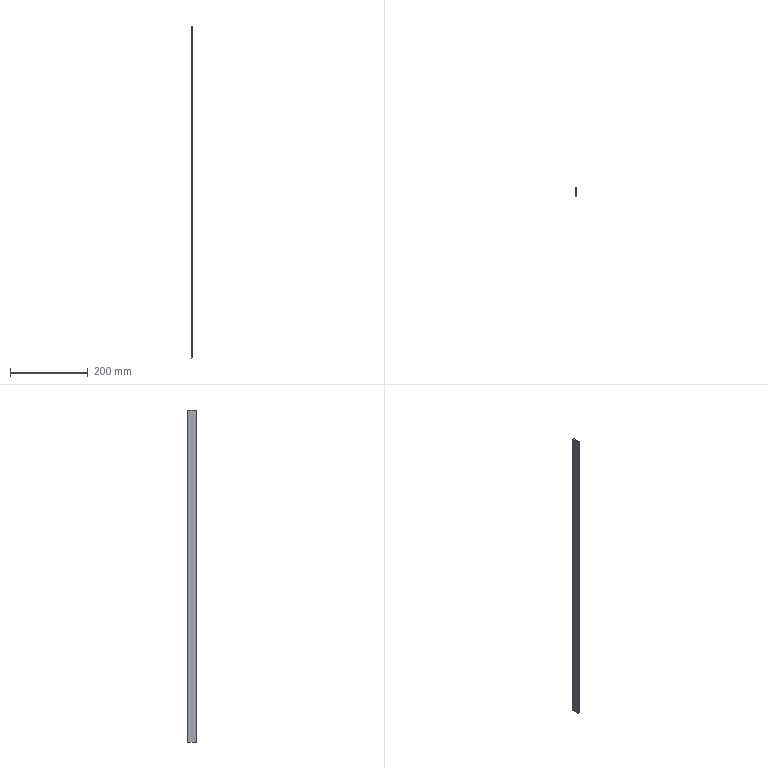Part | NX | features BREP 1 | 1 solid | 6 faces | box 4 x 22 x 853.93 mm | volume 75146 mm3 | plane 6
STEP:
#1=CARTESIAN_POINT('',(593.385,-607.17,1234.931));
#2=VERTEX_POINT('',#1);
#3=CARTESIAN_POINT('',(593.385,-629.17,1234.931));
#4=VERTEX_POINT('',#3);
#5=CARTESIAN_POINT('',(593.385,-618.17,1234.931));
#6=DIRECTION('',(0.,-1.,0.));
#7=VECTOR('',#6,1000.);
#8=LINE('',#5,#7);
#9=EDGE_CURVE('',#2,#4,#8,.T.);
#10=ORIENTED_EDGE('',*,*,#9,.F.);
#11=CARTESIAN_POINT('',(589.385,-607.17,1234.931));
#12=VERTEX_POINT('',#11);
#13=CARTESIAN_POINT('',(591.385,-607.17,1234.931));
#14=DIRECTION('',(1.,0.,0.000000042));
#15=VECTOR('',#14,1000.);
#16=LINE('',#13,#15);
#17=EDGE_CURVE('',#12,#2,#16,.T.);
#18=ORIENTED_EDGE('',*,*,#17,.F.);
#19=CARTESIAN_POINT('',(589.385,-629.17,1234.931));
#20=VERTEX_POINT('',#19);
#21=CARTESIAN_POINT('',(589.385,-618.17,1234.931));
#22=DIRECTION('',(0.,-1.,0.));
#23=VECTOR('',#22,1000.);
#24=LINE('',#21,#23);
#25=EDGE_CURVE('',#12,#20,#24,.T.);
#26=ORIENTED_EDGE('',*,*,#25,.T.);
#27=CARTESIAN_POINT('',(591.385,-629.17,1234.931));
#28=DIRECTION('',(1.,0.,0.000000042));
#29=VECTOR('',#28,1000.);
#30=LINE('',#27,#29);
#31=EDGE_CURVE('',#20,#4,#30,.T.);
#32=ORIENTED_EDGE('',*,*,#31,.T.);
#33=EDGE_LOOP('',(#10,#18,#26,#32));
#34=FACE_BOUND('',#33,.T.);
#35=CARTESIAN_POINT('',(589.385,-607.17,1234.931));
#36=DIRECTION('',(0.000000043,0.,-1.));
#37=DIRECTION('',(1.,0.,0.000000043));
#38=AXIS2_PLACEMENT_3D('',#35,#36,#37);
#39=PLANE('',#38);
#40=ADVANCED_FACE('',(#34),#39,.F.);
#41=CARTESIAN_POINT('',(589.385,-629.17,381.001));
#42=VERTEX_POINT('',#41);
#43=CARTESIAN_POINT('',(589.385,-629.17,807.966));
#44=DIRECTION('',(0.000000043,0.,-1.));
#45=VECTOR('',#44,1000.);
#46=LINE('',#43,#45);
#47=EDGE_CURVE('',#20,#42,#46,.T.);
#48=ORIENTED_EDGE('',*,*,#47,.T.);
#49=CARTESIAN_POINT('',(593.385,-629.17,381.001));
#50=VERTEX_POINT('',#49);
#51=CARTESIAN_POINT('',(591.385,-629.17,381.001));
#52=DIRECTION('',(1.,0.,0.000000043));
#53=VECTOR('',#52,1000.);
#54=LINE('',#51,#53);
#55=EDGE_CURVE('',#42,#50,#54,.T.);
#56=ORIENTED_EDGE('',*,*,#55,.T.);
#57=CARTESIAN_POINT('',(593.385,-629.17,807.966));
#58=DIRECTION('',(0.000000043,0.,-1.));
#59=VECTOR('',#58,1000.);
#60=LINE('',#57,#59);
#61=EDGE_CURVE('',#4,#50,#60,.T.);
#62=ORIENTED_EDGE('',*,*,#61,.F.);
#63=ORIENTED_EDGE('',*,*,#31,.F.);
#64=EDGE_LOOP('',(#48,#56,#62,#63));
#65=FACE_BOUND('',#64,.T.);
#66=CARTESIAN_POINT('',(591.385,-629.17,401.771));
#67=DIRECTION('',(0.,-1.,0.));
#68=DIRECTION('',(1.,0.,0.000000043));
#69=AXIS2_PLACEMENT_3D('',#66,#67,#68);
#70=PLANE('',#69);
#71=ADVANCED_FACE('',(#65),#70,.T.);
#72=ORIENTED_EDGE('',*,*,#61,.T.);
#73=CARTESIAN_POINT('',(593.385,-607.17,381.001));
#74=VERTEX_POINT('',#73);
#75=CARTESIAN_POINT('',(593.385,-618.17,381.001));
#76=DIRECTION('',(0.,1.,0.));
#77=VECTOR('',#76,1000.);
#78=LINE('',#75,#77);
#79=EDGE_CURVE('',#50,#74,#78,.T.);
#80=ORIENTED_EDGE('',*,*,#79,.T.);
#81=CARTESIAN_POINT('',(593.385,-607.17,807.966));
#82=DIRECTION('',(0.000000043,0.,-1.));
#83=VECTOR('',#82,1000.);
#84=LINE('',#81,#83);
#85=EDGE_CURVE('',#2,#74,#84,.T.);
#86=ORIENTED_EDGE('',*,*,#85,.F.);
#87=ORIENTED_EDGE('',*,*,#9,.T.);
#88=EDGE_LOOP('',(#72,#80,#86,#87));
#89=FACE_BOUND('',#88,.T.);
#90=CARTESIAN_POINT('',(593.385,-616.67,401.771));
#91=DIRECTION('',(1.,0.,0.000000043));
#92=DIRECTION('',(0.,-1.,-0.000003687));
#93=AXIS2_PLACEMENT_3D('',#90,#91,#92);
#94=PLANE('',#93);
#95=ADVANCED_FACE('',(#89),#94,.T.);
#96=ORIENTED_EDGE('',*,*,#17,.T.);
#97=ORIENTED_EDGE('',*,*,#85,.T.);
#98=CARTESIAN_POINT('',(589.385,-607.17,381.001));
#99=VERTEX_POINT('',#98);
#100=CARTESIAN_POINT('',(591.385,-607.17,381.001));
#101=DIRECTION('',(1.,0.,0.000000043));
#102=VECTOR('',#101,1000.);
#103=LINE('',#100,#102);
#104=EDGE_CURVE('',#99,#74,#103,.T.);
#105=ORIENTED_EDGE('',*,*,#104,.F.);
#106=CARTESIAN_POINT('',(589.385,-607.17,807.966));
#107=DIRECTION('',(-0.000000043,0.,1.));
#108=VECTOR('',#107,1000.);
#109=LINE('',#106,#108);
#110=EDGE_CURVE('',#99,#12,#109,.T.);
#111=ORIENTED_EDGE('',*,*,#110,.T.);
#112=EDGE_LOOP('',(#96,#97,#105,#111));
#113=FACE_BOUND('',#112,.T.);
#114=CARTESIAN_POINT('',(591.385,-607.17,401.771));
#115=DIRECTION('',(0.,-1.,0.));
#116=DIRECTION('',(1.,0.,0.000000043));
#117=AXIS2_PLACEMENT_3D('',#114,#115,#116);
#118=PLANE('',#117);
#119=ADVANCED_FACE('',(#113),#118,.F.);
#120=ORIENTED_EDGE('',*,*,#25,.F.);
#121=ORIENTED_EDGE('',*,*,#110,.F.);
#122=CARTESIAN_POINT('',(589.385,-618.17,381.001));
#123=DIRECTION('',(0.,1.,0.));
#124=VECTOR('',#123,1000.);
#125=LINE('',#122,#124);
#126=EDGE_CURVE('',#42,#99,#125,.T.);
#127=ORIENTED_EDGE('',*,*,#126,.F.);
#128=ORIENTED_EDGE('',*,*,#47,.F.);
#129=EDGE_LOOP('',(#120,#121,#127,#128));
#130=FACE_BOUND('',#129,.T.);
#131=CARTESIAN_POINT('',(589.385,-616.67,401.771));
#132=DIRECTION('',(1.,0.,0.000000043));
#133=DIRECTION('',(0.,-1.,-0.000003687));
#134=AXIS2_PLACEMENT_3D('',#131,#132,#133);
#135=PLANE('',#134);
#136=ADVANCED_FACE('',(#130),#135,.F.);
#137=ORIENTED_EDGE('',*,*,#126,.T.);
#138=ORIENTED_EDGE('',*,*,#104,.T.);
#139=ORIENTED_EDGE('',*,*,#79,.F.);
#140=ORIENTED_EDGE('',*,*,#55,.F.);
#141=EDGE_LOOP('',(#137,#138,#139,#140));
#142=FACE_BOUND('',#141,.T.);
#143=CARTESIAN_POINT('',(589.385,-629.17,381.001));
#144=DIRECTION('',(-0.000000043,0.,1.));
#145=DIRECTION('',(1.,0.,0.000000043));
#146=AXIS2_PLACEMENT_3D('',#143,#144,#145);
#147=PLANE('',#146);
#148=ADVANCED_FACE('',(#142),#147,.F.);
#149=CLOSED_SHELL('',(#40,#71,#95,#119,#136,#148));
#150=MANIFOLD_SOLID_BREP('',#149);
#151=(LENGTH_UNIT()NAMED_UNIT(*)SI_UNIT(.MILLI.,.METRE.));
#152=UNCERTAINTY_MEASURE_WITH_UNIT(LENGTH_MEASURE(0.00001),#151,'','');
#153=(NAMED_UNIT(*)PLANE_ANGLE_UNIT()SI_UNIT($,.RADIAN.));
#154=(NAMED_UNIT(*)SI_UNIT($,.STERADIAN.)SOLID_ANGLE_UNIT());
#155=(GEOMETRIC_REPRESENTATION_CONTEXT(3)GLOBAL_UNCERTAINTY_ASSIGNED_CONTEXT((#152))GLOBAL_UNIT_ASSIGNED_CONTEXT((#151,#153,#154))REPRESENTATION_CONTEXT('',''));
#156=ADVANCED_BREP_SHAPE_REPRESENTATION('',(#150),#155);